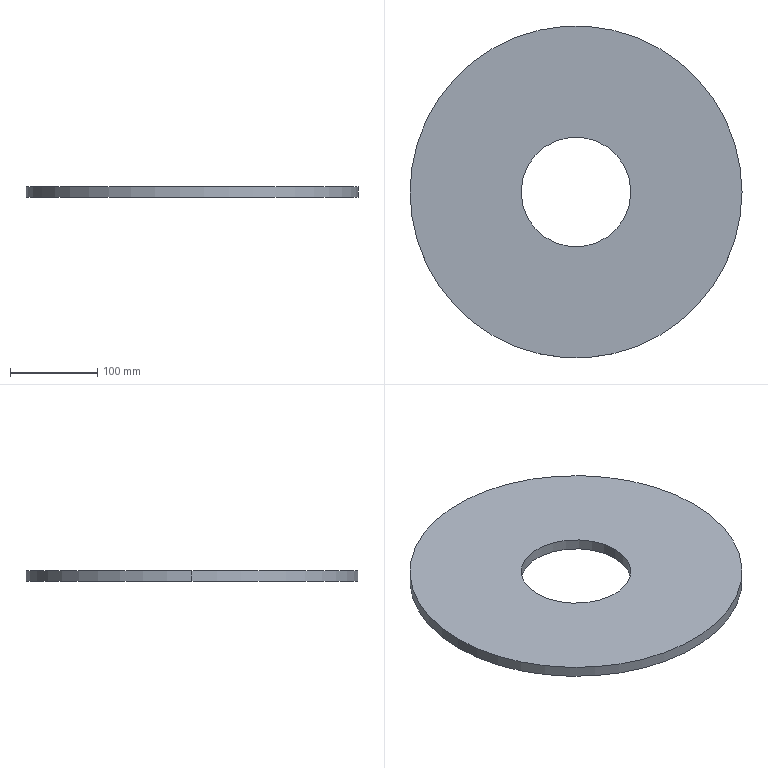Part | SolidWorks | features Extrusion 1 | 1 solid | 6 faces | box 380 x 380 x 12.5 mm | volume 1263016 mm3 | cylinder 4 | plane 2 | commonest cylinder face diameters 125.5 x2 380 x2
STEP:
#1=CARTESIAN_POINT('',(-62.75,0.,12.5));
#2=VERTEX_POINT('',#1);
#3=CARTESIAN_POINT('',(62.75,0.,12.5));
#4=VERTEX_POINT('',#3);
#5=CARTESIAN_POINT('',(0.,0.,12.5));
#6=DIRECTION('',(0.,0.,1.));
#7=DIRECTION('',(1.,0.,0.));
#8=AXIS2_PLACEMENT_3D('',#5,#6,#7);
#9=CIRCLE('',#8,62.75);
#10=EDGE_CURVE('',#2,#4,#9,.T.);
#11=ORIENTED_EDGE('',*,*,#10,.T.);
#12=CARTESIAN_POINT('',(62.75,0.,0.));
#13=VERTEX_POINT('',#12);
#14=CARTESIAN_POINT('',(62.75,0.,12.5));
#15=DIRECTION('',(0.,0.,-1.));
#16=VECTOR('',#15,1000.);
#17=LINE('',#14,#16);
#18=EDGE_CURVE('',#4,#13,#17,.T.);
#19=ORIENTED_EDGE('',*,*,#18,.T.);
#20=CARTESIAN_POINT('',(-62.75,0.,0.));
#21=VERTEX_POINT('',#20);
#22=CARTESIAN_POINT('',(0.,0.,0.));
#23=DIRECTION('',(0.,0.,1.));
#24=DIRECTION('',(1.,0.,0.));
#25=AXIS2_PLACEMENT_3D('',#22,#23,#24);
#26=CIRCLE('',#25,62.75);
#27=EDGE_CURVE('',#21,#13,#26,.T.);
#28=ORIENTED_EDGE('',*,*,#27,.F.);
#29=CARTESIAN_POINT('',(-62.75,0.,12.5));
#30=DIRECTION('',(0.,0.,-1.));
#31=VECTOR('',#30,1000.);
#32=LINE('',#29,#31);
#33=EDGE_CURVE('',#2,#21,#32,.T.);
#34=ORIENTED_EDGE('',*,*,#33,.F.);
#35=EDGE_LOOP('',(#11,#19,#28,#34));
#36=FACE_OUTER_BOUND('',#35,.T.);
#37=CARTESIAN_POINT('',(0.,0.,12.5));
#38=DIRECTION('',(0.,0.,-1.));
#39=DIRECTION('',(-1.,0.,0.));
#40=AXIS2_PLACEMENT_3D('',#37,#38,#39);
#41=CYLINDRICAL_SURFACE('',#40,62.75);
#42=ADVANCED_FACE('',(#36),#41,.F.);
#43=CARTESIAN_POINT('',(190.,0.,12.5));
#44=VERTEX_POINT('',#43);
#45=CARTESIAN_POINT('',(-190.,0.,12.5));
#46=VERTEX_POINT('',#45);
#47=CARTESIAN_POINT('',(0.,0.,12.5));
#48=DIRECTION('',(0.,0.,1.));
#49=DIRECTION('',(1.,0.,0.));
#50=AXIS2_PLACEMENT_3D('',#47,#48,#49);
#51=CIRCLE('',#50,190.);
#52=EDGE_CURVE('',#44,#46,#51,.T.);
#53=ORIENTED_EDGE('',*,*,#52,.F.);
#54=CARTESIAN_POINT('',(190.,0.,0.));
#55=VERTEX_POINT('',#54);
#56=CARTESIAN_POINT('',(190.,0.,12.5));
#57=DIRECTION('',(0.,0.,-1.));
#58=VECTOR('',#57,1000.);
#59=LINE('',#56,#58);
#60=EDGE_CURVE('',#44,#55,#59,.T.);
#61=ORIENTED_EDGE('',*,*,#60,.T.);
#62=CARTESIAN_POINT('',(-190.,0.,0.));
#63=VERTEX_POINT('',#62);
#64=CARTESIAN_POINT('',(0.,0.,0.));
#65=DIRECTION('',(0.,0.,1.));
#66=DIRECTION('',(1.,0.,0.));
#67=AXIS2_PLACEMENT_3D('',#64,#65,#66);
#68=CIRCLE('',#67,190.);
#69=EDGE_CURVE('',#55,#63,#68,.T.);
#70=ORIENTED_EDGE('',*,*,#69,.T.);
#71=CARTESIAN_POINT('',(-190.,0.,12.5));
#72=DIRECTION('',(0.,0.,-1.));
#73=VECTOR('',#72,1000.);
#74=LINE('',#71,#73);
#75=EDGE_CURVE('',#46,#63,#74,.T.);
#76=ORIENTED_EDGE('',*,*,#75,.F.);
#77=EDGE_LOOP('',(#53,#61,#70,#76));
#78=FACE_OUTER_BOUND('',#77,.T.);
#79=CARTESIAN_POINT('',(0.,0.,12.5));
#80=DIRECTION('',(0.,0.,-1.));
#81=DIRECTION('',(-1.,0.,0.));
#82=AXIS2_PLACEMENT_3D('',#79,#80,#81);
#83=CYLINDRICAL_SURFACE('',#82,190.);
#84=ADVANCED_FACE('',(#78),#83,.T.);
#85=CARTESIAN_POINT('',(0.,0.,12.5));
#86=DIRECTION('',(0.,0.,1.));
#87=DIRECTION('',(1.,0.,0.));
#88=AXIS2_PLACEMENT_3D('',#85,#86,#87);
#89=CIRCLE('',#88,190.);
#90=EDGE_CURVE('',#46,#44,#89,.T.);
#91=ORIENTED_EDGE('',*,*,#90,.T.);
#92=ORIENTED_EDGE('',*,*,#52,.T.);
#93=EDGE_LOOP('',(#91,#92));
#94=FACE_OUTER_BOUND('',#93,.T.);
#95=ORIENTED_EDGE('',*,*,#10,.F.);
#96=CARTESIAN_POINT('',(0.,0.,12.5));
#97=DIRECTION('',(0.,0.,1.));
#98=DIRECTION('',(1.,0.,0.));
#99=AXIS2_PLACEMENT_3D('',#96,#97,#98);
#100=CIRCLE('',#99,62.75);
#101=EDGE_CURVE('',#4,#2,#100,.T.);
#102=ORIENTED_EDGE('',*,*,#101,.F.);
#103=EDGE_LOOP('',(#95,#102));
#104=FACE_BOUND('',#103,.T.);
#105=CARTESIAN_POINT('',(0.,0.,12.5));
#106=DIRECTION('',(0.,0.,1.));
#107=DIRECTION('',(1.,0.,0.));
#108=AXIS2_PLACEMENT_3D('',#105,#106,#107);
#109=PLANE('',#108);
#110=ADVANCED_FACE('',(#94,#104),#109,.T.);
#111=CARTESIAN_POINT('',(0.,0.,0.));
#112=DIRECTION('',(0.,0.,1.));
#113=DIRECTION('',(1.,0.,0.));
#114=AXIS2_PLACEMENT_3D('',#111,#112,#113);
#115=CIRCLE('',#114,190.);
#116=EDGE_CURVE('',#63,#55,#115,.T.);
#117=ORIENTED_EDGE('',*,*,#116,.F.);
#118=ORIENTED_EDGE('',*,*,#69,.F.);
#119=EDGE_LOOP('',(#117,#118));
#120=FACE_OUTER_BOUND('',#119,.T.);
#121=ORIENTED_EDGE('',*,*,#27,.T.);
#122=CARTESIAN_POINT('',(0.,0.,0.));
#123=DIRECTION('',(0.,0.,1.));
#124=DIRECTION('',(1.,0.,0.));
#125=AXIS2_PLACEMENT_3D('',#122,#123,#124);
#126=CIRCLE('',#125,62.75);
#127=EDGE_CURVE('',#13,#21,#126,.T.);
#128=ORIENTED_EDGE('',*,*,#127,.T.);
#129=EDGE_LOOP('',(#121,#128));
#130=FACE_BOUND('',#129,.T.);
#131=CARTESIAN_POINT('',(0.,0.,0.));
#132=DIRECTION('',(0.,0.,1.));
#133=DIRECTION('',(1.,0.,0.));
#134=AXIS2_PLACEMENT_3D('',#131,#132,#133);
#135=PLANE('',#134);
#136=ADVANCED_FACE('',(#120,#130),#135,.F.);
#137=ORIENTED_EDGE('',*,*,#60,.F.);
#138=ORIENTED_EDGE('',*,*,#90,.F.);
#139=ORIENTED_EDGE('',*,*,#75,.T.);
#140=ORIENTED_EDGE('',*,*,#116,.T.);
#141=EDGE_LOOP('',(#137,#138,#139,#140));
#142=FACE_OUTER_BOUND('',#141,.T.);
#143=CARTESIAN_POINT('',(0.,0.,12.5));
#144=DIRECTION('',(0.,0.,-1.));
#145=DIRECTION('',(-1.,0.,0.));
#146=AXIS2_PLACEMENT_3D('',#143,#144,#145);
#147=CYLINDRICAL_SURFACE('',#146,190.);
#148=ADVANCED_FACE('',(#142),#147,.T.);
#149=ORIENTED_EDGE('',*,*,#18,.F.);
#150=ORIENTED_EDGE('',*,*,#101,.T.);
#151=ORIENTED_EDGE('',*,*,#33,.T.);
#152=ORIENTED_EDGE('',*,*,#127,.F.);
#153=EDGE_LOOP('',(#149,#150,#151,#152));
#154=FACE_OUTER_BOUND('',#153,.T.);
#155=CARTESIAN_POINT('',(0.,0.,12.5));
#156=DIRECTION('',(0.,0.,-1.));
#157=DIRECTION('',(-1.,0.,0.));
#158=AXIS2_PLACEMENT_3D('',#155,#156,#157);
#159=CYLINDRICAL_SURFACE('',#158,62.75);
#160=ADVANCED_FACE('',(#154),#159,.F.);
#161=CLOSED_SHELL('',(#42,#84,#110,#136,#148,#160));
#162=MANIFOLD_SOLID_BREP('',#161);
#163=CARTESIAN_POINT('',(0.,0.,0.));
#164=DIRECTION('',(0.,0.,1.));
#165=DIRECTION('',(1.,0.,0.));
#166=AXIS2_PLACEMENT_3D('',#163,#164,#165);
#167=(LENGTH_UNIT()NAMED_UNIT(*)SI_UNIT(.MILLI.,.METRE.));
#168=UNCERTAINTY_MEASURE_WITH_UNIT(LENGTH_MEASURE(0.00001),#167,'','');
#169=(NAMED_UNIT(*)PLANE_ANGLE_UNIT()SI_UNIT($,.RADIAN.));
#170=(NAMED_UNIT(*)SI_UNIT($,.STERADIAN.)SOLID_ANGLE_UNIT());
#171=(GEOMETRIC_REPRESENTATION_CONTEXT(3)GLOBAL_UNCERTAINTY_ASSIGNED_CONTEXT((#168))GLOBAL_UNIT_ASSIGNED_CONTEXT((#167,#169,#170))REPRESENTATION_CONTEXT('',''));
#172=ADVANCED_BREP_SHAPE_REPRESENTATION('',(#162,#166),#171);